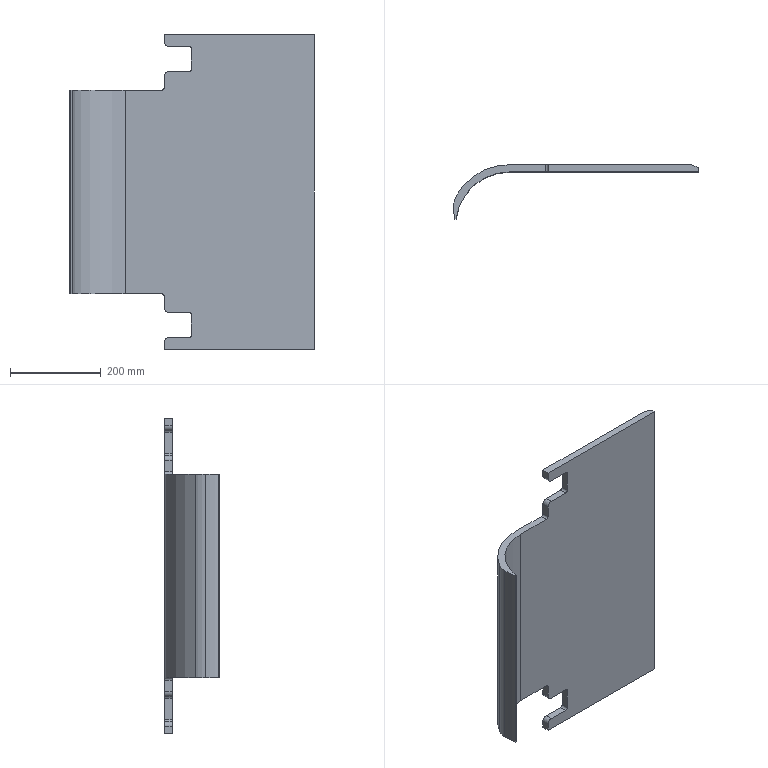Part | SolidWorks | features ICE 2, Extrusion 1 | 1 solid | 33 faces | box 540.8 x 120 x 696 mm | volume 5367152 mm3 | plane 19 | cylinder 14 | commonest cylinder face diameters 10 x6 20 x4 100 x1 236 x1 245.6 x1 268 x1
STEP:
#1=CARTESIAN_POINT('',(418.,9.,-348.));
#2=VERTEX_POINT('',#1);
#3=CARTESIAN_POINT('',(403.,16.,-348.));
#4=VERTEX_POINT('',#3);
#5=CARTESIAN_POINT('',(418.,9.,-348.));
#6=DIRECTION('',(-0.9062,0.4229,0.));
#7=VECTOR('',#6,1000.);
#8=LINE('',#5,#7);
#9=EDGE_CURVE('',#2,#4,#8,.T.);
#10=ORIENTED_EDGE('',*,*,#9,.T.);
#11=CARTESIAN_POINT('',(403.,16.,348.));
#12=VERTEX_POINT('',#11);
#13=CARTESIAN_POINT('',(403.,16.,348.));
#14=DIRECTION('',(0.,0.,-1.));
#15=VECTOR('',#14,1000.);
#16=LINE('',#13,#15);
#17=EDGE_CURVE('',#12,#4,#16,.T.);
#18=ORIENTED_EDGE('',*,*,#17,.F.);
#19=CARTESIAN_POINT('',(418.,9.,348.));
#20=VERTEX_POINT('',#19);
#21=CARTESIAN_POINT('',(418.,9.,348.));
#22=DIRECTION('',(-0.9062,0.4229,0.));
#23=VECTOR('',#22,1000.);
#24=LINE('',#21,#23);
#25=EDGE_CURVE('',#20,#12,#24,.T.);
#26=ORIENTED_EDGE('',*,*,#25,.F.);
#27=CARTESIAN_POINT('',(418.,9.,348.));
#28=DIRECTION('',(0.,0.,-1.));
#29=VECTOR('',#28,1000.);
#30=LINE('',#27,#29);
#31=EDGE_CURVE('',#20,#2,#30,.T.);
#32=ORIENTED_EDGE('',*,*,#31,.T.);
#33=EDGE_LOOP('',(#10,#18,#26,#32));
#34=FACE_OUTER_BOUND('',#33,.T.);
#35=CARTESIAN_POINT('',(418.,9.,348.));
#36=DIRECTION('',(-0.4229,-0.9062,0.));
#37=DIRECTION('',(0.9062,-0.4229,0.));
#38=AXIS2_PLACEMENT_3D('',#35,#36,#37);
#39=PLANE('',#38);
#40=ADVANCED_FACE('',(#34),#39,.F.);
#41=CARTESIAN_POINT('',(0.,16.,225.));
#42=VERTEX_POINT('',#41);
#43=CARTESIAN_POINT('',(0.,16.,-225.));
#44=VERTEX_POINT('',#43);
#45=CARTESIAN_POINT('',(0.,16.,348.));
#46=DIRECTION('',(0.,0.,-1.));
#47=VECTOR('',#46,1000.);
#48=LINE('',#45,#47);
#49=EDGE_CURVE('',#42,#44,#48,.T.);
#50=ORIENTED_EDGE('',*,*,#49,.F.);
#51=CARTESIAN_POINT('',(81.,16.,225.));
#52=VERTEX_POINT('',#51);
#53=CARTESIAN_POINT('',(81.,16.,225.));
#54=DIRECTION('',(-1.,0.,0.));
#55=VECTOR('',#54,1000.);
#56=LINE('',#53,#55);
#57=EDGE_CURVE('',#52,#42,#56,.T.);
#58=ORIENTED_EDGE('',*,*,#57,.F.);
#59=CARTESIAN_POINT('',(86.,16.,230.));
#60=VERTEX_POINT('',#59);
#61=CARTESIAN_POINT('',(81.,16.,230.));
#62=DIRECTION('',(0.,1.,0.));
#63=DIRECTION('',(0.,0.,1.));
#64=AXIS2_PLACEMENT_3D('',#61,#62,#63);
#65=CIRCLE('',#64,5.);
#66=EDGE_CURVE('',#60,#52,#65,.T.);
#67=ORIENTED_EDGE('',*,*,#66,.F.);
#68=CARTESIAN_POINT('',(86.,16.,256.));
#69=VERTEX_POINT('',#68);
#70=CARTESIAN_POINT('',(86.,16.,256.));
#71=DIRECTION('',(0.,0.,-1.));
#72=VECTOR('',#71,1000.);
#73=LINE('',#70,#72);
#74=EDGE_CURVE('',#69,#60,#73,.T.);
#75=ORIENTED_EDGE('',*,*,#74,.F.);
#76=CARTESIAN_POINT('',(96.,16.,266.));
#77=VERTEX_POINT('',#76);
#78=CARTESIAN_POINT('',(96.,16.,256.));
#79=DIRECTION('',(0.,-1.,0.));
#80=DIRECTION('',(0.,0.,-1.));
#81=AXIS2_PLACEMENT_3D('',#78,#79,#80);
#82=CIRCLE('',#81,10.);
#83=EDGE_CURVE('',#77,#69,#82,.T.);
#84=ORIENTED_EDGE('',*,*,#83,.F.);
#85=CARTESIAN_POINT('',(141.,16.,266.));
#86=VERTEX_POINT('',#85);
#87=CARTESIAN_POINT('',(141.,16.,266.));
#88=DIRECTION('',(-1.,0.,0.));
#89=VECTOR('',#88,1000.);
#90=LINE('',#87,#89);
#91=EDGE_CURVE('',#86,#77,#90,.T.);
#92=ORIENTED_EDGE('',*,*,#91,.F.);
#93=CARTESIAN_POINT('',(146.,16.,271.));
#94=VERTEX_POINT('',#93);
#95=CARTESIAN_POINT('',(141.,16.,271.));
#96=DIRECTION('',(0.,1.,0.));
#97=DIRECTION('',(0.,0.,-1.));
#98=AXIS2_PLACEMENT_3D('',#95,#96,#97);
#99=CIRCLE('',#98,5.);
#100=EDGE_CURVE('',#94,#86,#99,.T.);
#101=ORIENTED_EDGE('',*,*,#100,.F.);
#102=CARTESIAN_POINT('',(146.,16.,317.));
#103=VERTEX_POINT('',#102);
#104=CARTESIAN_POINT('',(146.,16.,317.));
#105=DIRECTION('',(0.,0.,-1.));
#106=VECTOR('',#105,1000.);
#107=LINE('',#104,#106);
#108=EDGE_CURVE('',#103,#94,#107,.T.);
#109=ORIENTED_EDGE('',*,*,#108,.F.);
#110=CARTESIAN_POINT('',(141.,16.,322.));
#111=VERTEX_POINT('',#110);
#112=CARTESIAN_POINT('',(141.,16.,317.));
#113=DIRECTION('',(0.,1.,0.));
#114=DIRECTION('',(0.,0.,-1.));
#115=AXIS2_PLACEMENT_3D('',#112,#113,#114);
#116=CIRCLE('',#115,5.);
#117=EDGE_CURVE('',#111,#103,#116,.T.);
#118=ORIENTED_EDGE('',*,*,#117,.F.);
#119=CARTESIAN_POINT('',(96.,16.,322.));
#120=VERTEX_POINT('',#119);
#121=CARTESIAN_POINT('',(96.,16.,322.));
#122=DIRECTION('',(1.,0.,0.));
#123=VECTOR('',#122,1000.);
#124=LINE('',#121,#123);
#125=EDGE_CURVE('',#120,#111,#124,.T.);
#126=ORIENTED_EDGE('',*,*,#125,.F.);
#127=CARTESIAN_POINT('',(86.,16.,332.));
#128=VERTEX_POINT('',#127);
#129=CARTESIAN_POINT('',(96.,16.,332.));
#130=DIRECTION('',(0.,-1.,0.));
#131=DIRECTION('',(0.,0.,1.));
#132=AXIS2_PLACEMENT_3D('',#129,#130,#131);
#133=CIRCLE('',#132,10.);
#134=EDGE_CURVE('',#128,#120,#133,.T.);
#135=ORIENTED_EDGE('',*,*,#134,.F.);
#136=CARTESIAN_POINT('',(86.,16.,348.));
#137=VERTEX_POINT('',#136);
#138=CARTESIAN_POINT('',(86.,16.,332.));
#139=DIRECTION('',(0.,0.,-1.));
#140=VECTOR('',#139,1000.);
#141=LINE('',#138,#140);
#142=EDGE_CURVE('',#137,#128,#141,.T.);
#143=ORIENTED_EDGE('',*,*,#142,.F.);
#144=CARTESIAN_POINT('',(0.,16.,348.));
#145=DIRECTION('',(-1.,0.,0.));
#146=VECTOR('',#145,1000.);
#147=LINE('',#144,#146);
#148=EDGE_CURVE('',#12,#137,#147,.T.);
#149=ORIENTED_EDGE('',*,*,#148,.F.);
#150=ORIENTED_EDGE('',*,*,#17,.T.);
#151=CARTESIAN_POINT('',(86.,16.,-348.));
#152=VERTEX_POINT('',#151);
#153=CARTESIAN_POINT('',(0.,16.,-348.));
#154=DIRECTION('',(-1.,0.,0.));
#155=VECTOR('',#154,1000.);
#156=LINE('',#153,#155);
#157=EDGE_CURVE('',#4,#152,#156,.T.);
#158=ORIENTED_EDGE('',*,*,#157,.T.);
#159=CARTESIAN_POINT('',(86.,16.,-332.));
#160=VERTEX_POINT('',#159);
#161=CARTESIAN_POINT('',(86.,16.,-332.));
#162=DIRECTION('',(0.,0.,-1.));
#163=VECTOR('',#162,1000.);
#164=LINE('',#161,#163);
#165=EDGE_CURVE('',#160,#152,#164,.T.);
#166=ORIENTED_EDGE('',*,*,#165,.F.);
#167=CARTESIAN_POINT('',(96.,16.,-322.));
#168=VERTEX_POINT('',#167);
#169=CARTESIAN_POINT('',(96.,16.,-332.));
#170=DIRECTION('',(0.,-1.,0.));
#171=DIRECTION('',(0.,0.,-1.));
#172=AXIS2_PLACEMENT_3D('',#169,#170,#171);
#173=CIRCLE('',#172,10.);
#174=EDGE_CURVE('',#168,#160,#173,.T.);
#175=ORIENTED_EDGE('',*,*,#174,.F.);
#176=CARTESIAN_POINT('',(141.,16.,-322.));
#177=VERTEX_POINT('',#176);
#178=CARTESIAN_POINT('',(96.,16.,-322.));
#179=DIRECTION('',(-1.,0.,0.));
#180=VECTOR('',#179,1000.);
#181=LINE('',#178,#180);
#182=EDGE_CURVE('',#177,#168,#181,.T.);
#183=ORIENTED_EDGE('',*,*,#182,.F.);
#184=CARTESIAN_POINT('',(146.,16.,-317.));
#185=VERTEX_POINT('',#184);
#186=CARTESIAN_POINT('',(141.,16.,-317.));
#187=DIRECTION('',(0.,1.,0.));
#188=DIRECTION('',(0.,0.,1.));
#189=AXIS2_PLACEMENT_3D('',#186,#187,#188);
#190=CIRCLE('',#189,5.);
#191=EDGE_CURVE('',#185,#177,#190,.T.);
#192=ORIENTED_EDGE('',*,*,#191,.F.);
#193=CARTESIAN_POINT('',(146.,16.,-271.));
#194=VERTEX_POINT('',#193);
#195=CARTESIAN_POINT('',(146.,16.,-317.));
#196=DIRECTION('',(0.,0.,-1.));
#197=VECTOR('',#196,1000.);
#198=LINE('',#195,#197);
#199=EDGE_CURVE('',#194,#185,#198,.T.);
#200=ORIENTED_EDGE('',*,*,#199,.F.);
#201=CARTESIAN_POINT('',(141.,16.,-266.));
#202=VERTEX_POINT('',#201);
#203=CARTESIAN_POINT('',(141.,16.,-271.));
#204=DIRECTION('',(0.,1.,0.));
#205=DIRECTION('',(0.,0.,1.));
#206=AXIS2_PLACEMENT_3D('',#203,#204,#205);
#207=CIRCLE('',#206,5.);
#208=EDGE_CURVE('',#202,#194,#207,.T.);
#209=ORIENTED_EDGE('',*,*,#208,.F.);
#210=CARTESIAN_POINT('',(96.,16.,-266.));
#211=VERTEX_POINT('',#210);
#212=CARTESIAN_POINT('',(141.,16.,-266.));
#213=DIRECTION('',(1.,0.,0.));
#214=VECTOR('',#213,1000.);
#215=LINE('',#212,#214);
#216=EDGE_CURVE('',#211,#202,#215,.T.);
#217=ORIENTED_EDGE('',*,*,#216,.F.);
#218=CARTESIAN_POINT('',(86.,16.,-256.));
#219=VERTEX_POINT('',#218);
#220=CARTESIAN_POINT('',(96.,16.,-256.));
#221=DIRECTION('',(0.,-1.,0.));
#222=DIRECTION('',(0.,0.,1.));
#223=AXIS2_PLACEMENT_3D('',#220,#221,#222);
#224=CIRCLE('',#223,10.);
#225=EDGE_CURVE('',#219,#211,#224,.T.);
#226=ORIENTED_EDGE('',*,*,#225,.F.);
#227=CARTESIAN_POINT('',(86.,16.,-230.));
#228=VERTEX_POINT('',#227);
#229=CARTESIAN_POINT('',(86.,16.,-256.));
#230=DIRECTION('',(0.,0.,-1.));
#231=VECTOR('',#230,1000.);
#232=LINE('',#229,#231);
#233=EDGE_CURVE('',#228,#219,#232,.T.);
#234=ORIENTED_EDGE('',*,*,#233,.F.);
#235=CARTESIAN_POINT('',(81.,16.,-225.));
#236=VERTEX_POINT('',#235);
#237=CARTESIAN_POINT('',(81.,16.,-230.));
#238=DIRECTION('',(0.,1.,0.));
#239=DIRECTION('',(0.,0.,-1.));
#240=AXIS2_PLACEMENT_3D('',#237,#238,#239);
#241=CIRCLE('',#240,5.);
#242=EDGE_CURVE('',#236,#228,#241,.T.);
#243=ORIENTED_EDGE('',*,*,#242,.F.);
#244=CARTESIAN_POINT('',(81.,16.,-225.));
#245=DIRECTION('',(1.,0.,0.));
#246=VECTOR('',#245,1000.);
#247=LINE('',#244,#246);
#248=EDGE_CURVE('',#44,#236,#247,.T.);
#249=ORIENTED_EDGE('',*,*,#248,.F.);
#250=EDGE_LOOP('',(#50,#58,#67,#75,#84,#92,#101,#109,#118,#126,#135,#143,#149,#150,#158,#166,#175,#183,#192,#200,#209,#217,#226,#234,#243,#249));
#251=FACE_OUTER_BOUND('',#250,.T.);
#252=CARTESIAN_POINT('',(0.,16.,348.));
#253=DIRECTION('',(0.,-1.,0.));
#254=DIRECTION('',(1.,0.,0.));
#255=AXIS2_PLACEMENT_3D('',#252,#253,#254);
#256=PLANE('',#255);
#257=ADVANCED_FACE('',(#251),#256,.F.);
#258=CARTESIAN_POINT('',(-116.034,-50.976,-225.));
#259=VERTEX_POINT('',#258);
#260=CARTESIAN_POINT('',(0.,-118.,-225.));
#261=DIRECTION('',(0.,0.,1.));
#262=DIRECTION('',(1.,0.,0.));
#263=AXIS2_PLACEMENT_3D('',#260,#261,#262);
#264=CIRCLE('',#263,134.);
#265=EDGE_CURVE('',#44,#259,#264,.T.);
#266=ORIENTED_EDGE('',*,*,#265,.T.);
#267=CARTESIAN_POINT('',(-116.034,-50.976,225.));
#268=VERTEX_POINT('',#267);
#269=CARTESIAN_POINT('',(-116.034,-50.976,-348.));
#270=DIRECTION('',(0.,0.,1.));
#271=VECTOR('',#270,1000.);
#272=LINE('',#269,#271);
#273=EDGE_CURVE('',#259,#268,#272,.T.);
#274=ORIENTED_EDGE('',*,*,#273,.T.);
#275=CARTESIAN_POINT('',(0.,-118.,225.));
#276=DIRECTION('',(0.,0.,-1.));
#277=DIRECTION('',(-1.,0.,0.));
#278=AXIS2_PLACEMENT_3D('',#275,#276,#277);
#279=CIRCLE('',#278,134.);
#280=EDGE_CURVE('',#268,#42,#279,.T.);
#281=ORIENTED_EDGE('',*,*,#280,.T.);
#282=ORIENTED_EDGE('',*,*,#49,.T.);
#283=EDGE_LOOP('',(#266,#274,#281,#282));
#284=FACE_OUTER_BOUND('',#283,.T.);
#285=CARTESIAN_POINT('',(0.,-118.,348.));
#286=DIRECTION('',(0.,0.,-1.));
#287=DIRECTION('',(-1.,0.,0.));
#288=AXIS2_PLACEMENT_3D('',#285,#286,#287);
#289=CYLINDRICAL_SURFACE('',#288,134.);
#290=ADVANCED_FACE('',(#284),#289,.T.);
#291=CARTESIAN_POINT('',(-117.167,-104.,225.));
#292=VERTEX_POINT('',#291);
#293=CARTESIAN_POINT('',(-120.306,-103.625,225.));
#294=VERTEX_POINT('',#293);
#295=CARTESIAN_POINT('',(-117.167,-104.,225.));
#296=DIRECTION('',(-0.9929,0.1186,0.));
#297=VECTOR('',#296,1000.);
#298=LINE('',#295,#297);
#299=EDGE_CURVE('',#292,#294,#298,.T.);
#300=ORIENTED_EDGE('',*,*,#299,.T.);
#301=CARTESIAN_POINT('',(-120.306,-103.625,-225.));
#302=VERTEX_POINT('',#301);
#303=CARTESIAN_POINT('',(-120.306,-103.625,-348.));
#304=DIRECTION('',(0.,0.,1.));
#305=VECTOR('',#304,1000.);
#306=LINE('',#303,#305);
#307=EDGE_CURVE('',#302,#294,#306,.T.);
#308=ORIENTED_EDGE('',*,*,#307,.F.);
#309=CARTESIAN_POINT('',(-117.167,-104.,-225.));
#310=VERTEX_POINT('',#309);
#311=CARTESIAN_POINT('',(-117.167,-104.,-225.));
#312=DIRECTION('',(0.9929,-0.1186,0.));
#313=VECTOR('',#312,1000.);
#314=LINE('',#311,#313);
#315=EDGE_CURVE('',#302,#310,#314,.T.);
#316=ORIENTED_EDGE('',*,*,#315,.T.);
#317=CARTESIAN_POINT('',(-117.167,-104.,348.));
#318=DIRECTION('',(0.,0.,-1.));
#319=VECTOR('',#318,1000.);
#320=LINE('',#317,#319);
#321=EDGE_CURVE('',#292,#310,#320,.T.);
#322=ORIENTED_EDGE('',*,*,#321,.F.);
#323=EDGE_LOOP('',(#300,#308,#316,#322));
#324=FACE_OUTER_BOUND('',#323,.T.);
#325=CARTESIAN_POINT('',(-117.167,-104.,348.));
#326=DIRECTION('',(0.1186,0.9929,0.));
#327=DIRECTION('',(-0.9929,0.1186,0.));
#328=AXIS2_PLACEMENT_3D('',#325,#326,#327);
#329=PLANE('',#328);
#330=ADVANCED_FACE('',(#324),#329,.F.);
#331=CARTESIAN_POINT('',(0.,0.,225.));
#332=VERTEX_POINT('',#331);
#333=CARTESIAN_POINT('',(0.,0.,-225.));
#334=VERTEX_POINT('',#333);
#335=CARTESIAN_POINT('',(0.,0.,348.));
#336=DIRECTION('',(0.,0.,-1.));
#337=VECTOR('',#336,1000.);
#338=LINE('',#335,#337);
#339=EDGE_CURVE('',#332,#334,#338,.T.);
#340=ORIENTED_EDGE('',*,*,#339,.F.);
#341=CARTESIAN_POINT('',(0.,-118.,225.));
#342=DIRECTION('',(0.,0.,1.));
#343=DIRECTION('',(-1.,0.,0.));
#344=AXIS2_PLACEMENT_3D('',#341,#342,#343);
#345=CIRCLE('',#344,118.);
#346=EDGE_CURVE('',#332,#292,#345,.T.);
#347=ORIENTED_EDGE('',*,*,#346,.T.);
#348=ORIENTED_EDGE('',*,*,#321,.T.);
#349=CARTESIAN_POINT('',(0.,-118.,-225.));
#350=DIRECTION('',(0.,0.,-1.));
#351=DIRECTION('',(1.,0.,0.));
#352=AXIS2_PLACEMENT_3D('',#349,#350,#351);
#353=CIRCLE('',#352,118.);
#354=EDGE_CURVE('',#310,#334,#353,.T.);
#355=ORIENTED_EDGE('',*,*,#354,.T.);
#356=EDGE_LOOP('',(#340,#347,#348,#355));
#357=FACE_OUTER_BOUND('',#356,.T.);
#358=CARTESIAN_POINT('',(0.,-118.,348.));
#359=DIRECTION('',(0.,0.,-1.));
#360=DIRECTION('',(-1.,0.,0.));
#361=AXIS2_PLACEMENT_3D('',#358,#359,#360);
#362=CYLINDRICAL_SURFACE('',#361,118.);
#363=ADVANCED_FACE('',(#357),#362,.F.);
#364=CARTESIAN_POINT('',(86.,0.,230.));
#365=VERTEX_POINT('',#364);
#366=CARTESIAN_POINT('',(81.,0.,225.));
#367=VERTEX_POINT('',#366);
#368=CARTESIAN_POINT('',(81.,0.,230.));
#369=DIRECTION('',(0.,1.,0.));
#370=DIRECTION('',(0.,0.,1.));
#371=AXIS2_PLACEMENT_3D('',#368,#369,#370);
#372=CIRCLE('',#371,5.);
#373=EDGE_CURVE('',#365,#367,#372,.T.);
#374=ORIENTED_EDGE('',*,*,#373,.T.);
#375=CARTESIAN_POINT('',(0.,0.,225.));
#376=DIRECTION('',(-1.,0.,0.));
#377=VECTOR('',#376,1000.);
#378=LINE('',#375,#377);
#379=EDGE_CURVE('',#367,#332,#378,.T.);
#380=ORIENTED_EDGE('',*,*,#379,.T.);
#381=ORIENTED_EDGE('',*,*,#339,.T.);
#382=CARTESIAN_POINT('',(81.,0.,-225.));
#383=VERTEX_POINT('',#382);
#384=CARTESIAN_POINT('',(0.,0.,-225.));
#385=DIRECTION('',(1.,0.,0.));
#386=VECTOR('',#385,1000.);
#387=LINE('',#384,#386);
#388=EDGE_CURVE('',#334,#383,#387,.T.);
#389=ORIENTED_EDGE('',*,*,#388,.T.);
#390=CARTESIAN_POINT('',(86.,0.,-230.));
#391=VERTEX_POINT('',#390);
#392=CARTESIAN_POINT('',(81.,0.,-230.));
#393=DIRECTION('',(0.,1.,0.));
#394=DIRECTION('',(0.,0.,1.));
#395=AXIS2_PLACEMENT_3D('',#392,#393,#394);
#396=CIRCLE('',#395,5.);
#397=EDGE_CURVE('',#383,#391,#396,.T.);
#398=ORIENTED_EDGE('',*,*,#397,.T.);
#399=CARTESIAN_POINT('',(86.,0.,-256.));
#400=VERTEX_POINT('',#399);
#401=CARTESIAN_POINT('',(86.,0.,348.));
#402=DIRECTION('',(0.,0.,-1.));
#403=VECTOR('',#402,1000.);
#404=LINE('',#401,#403);
#405=EDGE_CURVE('',#391,#400,#404,.T.);
#406=ORIENTED_EDGE('',*,*,#405,.T.);
#407=CARTESIAN_POINT('',(96.,0.,-266.));
#408=VERTEX_POINT('',#407);
#409=CARTESIAN_POINT('',(96.,0.,-256.));
#410=DIRECTION('',(0.,-1.,0.));
#411=DIRECTION('',(0.,0.,1.));
#412=AXIS2_PLACEMENT_3D('',#409,#410,#411);
#413=CIRCLE('',#412,10.);
#414=EDGE_CURVE('',#400,#408,#413,.T.);
#415=ORIENTED_EDGE('',*,*,#414,.T.);
#416=CARTESIAN_POINT('',(141.,0.,-266.));
#417=VERTEX_POINT('',#416);
#418=CARTESIAN_POINT('',(0.,0.,-266.));
#419=DIRECTION('',(1.,0.,0.));
#420=VECTOR('',#419,1000.);
#421=LINE('',#418,#420);
#422=EDGE_CURVE('',#408,#417,#421,.T.);
#423=ORIENTED_EDGE('',*,*,#422,.T.);
#424=CARTESIAN_POINT('',(146.,0.,-271.));
#425=VERTEX_POINT('',#424);
#426=CARTESIAN_POINT('',(141.,0.,-271.));
#427=DIRECTION('',(0.,1.,0.));
#428=DIRECTION('',(0.,0.,1.));
#429=AXIS2_PLACEMENT_3D('',#426,#427,#428);
#430=CIRCLE('',#429,5.);
#431=EDGE_CURVE('',#417,#425,#430,.T.);
#432=ORIENTED_EDGE('',*,*,#431,.T.);
#433=CARTESIAN_POINT('',(146.,0.,-317.));
#434=VERTEX_POINT('',#433);
#435=CARTESIAN_POINT('',(146.,0.,348.));
#436=DIRECTION('',(0.,0.,-1.));
#437=VECTOR('',#436,1000.);
#438=LINE('',#435,#437);
#439=EDGE_CURVE('',#425,#434,#438,.T.);
#440=ORIENTED_EDGE('',*,*,#439,.T.);
#441=CARTESIAN_POINT('',(141.,0.,-322.));
#442=VERTEX_POINT('',#441);
#443=CARTESIAN_POINT('',(141.,0.,-317.));
#444=DIRECTION('',(0.,1.,0.));
#445=DIRECTION('',(0.,0.,1.));
#446=AXIS2_PLACEMENT_3D('',#443,#444,#445);
#447=CIRCLE('',#446,5.);
#448=EDGE_CURVE('',#434,#442,#447,.T.);
#449=ORIENTED_EDGE('',*,*,#448,.T.);
#450=CARTESIAN_POINT('',(96.,0.,-322.));
#451=VERTEX_POINT('',#450);
#452=CARTESIAN_POINT('',(0.,0.,-322.));
#453=DIRECTION('',(-1.,0.,0.));
#454=VECTOR('',#453,1000.);
#455=LINE('',#452,#454);
#456=EDGE_CURVE('',#442,#451,#455,.T.);
#457=ORIENTED_EDGE('',*,*,#456,.T.);
#458=CARTESIAN_POINT('',(86.,0.,-332.));
#459=VERTEX_POINT('',#458);
#460=CARTESIAN_POINT('',(96.,0.,-332.));
#461=DIRECTION('',(0.,-1.,0.));
#462=DIRECTION('',(0.,0.,1.));
#463=AXIS2_PLACEMENT_3D('',#460,#461,#462);
#464=CIRCLE('',#463,10.);
#465=EDGE_CURVE('',#451,#459,#464,.T.);
#466=ORIENTED_EDGE('',*,*,#465,.T.);
#467=CARTESIAN_POINT('',(86.,0.,-348.));
#468=VERTEX_POINT('',#467);
#469=CARTESIAN_POINT('',(86.,0.,348.));
#470=DIRECTION('',(0.,0.,-1.));
#471=VECTOR('',#470,1000.);
#472=LINE('',#469,#471);
#473=EDGE_CURVE('',#459,#468,#472,.T.);
#474=ORIENTED_EDGE('',*,*,#473,.T.);
#475=CARTESIAN_POINT('',(418.,0.,-348.));
#476=VERTEX_POINT('',#475);
#477=CARTESIAN_POINT('',(0.,0.,-348.));
#478=DIRECTION('',(1.,0.,0.));
#479=VECTOR('',#478,1000.);
#480=LINE('',#477,#479);
#481=EDGE_CURVE('',#468,#476,#480,.T.);
#482=ORIENTED_EDGE('',*,*,#481,.T.);
#483=CARTESIAN_POINT('',(418.,0.,348.));
#484=VERTEX_POINT('',#483);
#485=CARTESIAN_POINT('',(418.,0.,348.));
#486=DIRECTION('',(0.,0.,-1.));
#487=VECTOR('',#486,1000.);
#488=LINE('',#485,#487);
#489=EDGE_CURVE('',#484,#476,#488,.T.);
#490=ORIENTED_EDGE('',*,*,#489,.F.);
#491=CARTESIAN_POINT('',(86.,0.,348.));
#492=VERTEX_POINT('',#491);
#493=CARTESIAN_POINT('',(0.,0.,348.));
#494=DIRECTION('',(1.,0.,0.));
#495=VECTOR('',#494,1000.);
#496=LINE('',#493,#495);
#497=EDGE_CURVE('',#492,#484,#496,.T.);
#498=ORIENTED_EDGE('',*,*,#497,.F.);
#499=CARTESIAN_POINT('',(86.,0.,332.));
#500=VERTEX_POINT('',#499);
#501=CARTESIAN_POINT('',(86.,0.,348.));
#502=DIRECTION('',(0.,0.,-1.));
#503=VECTOR('',#502,1000.);
#504=LINE('',#501,#503);
#505=EDGE_CURVE('',#492,#500,#504,.T.);
#506=ORIENTED_EDGE('',*,*,#505,.T.);
#507=CARTESIAN_POINT('',(96.,0.,322.));
#508=VERTEX_POINT('',#507);
#509=CARTESIAN_POINT('',(96.,0.,332.));
#510=DIRECTION('',(0.,-1.,0.));
#511=DIRECTION('',(0.,0.,1.));
#512=AXIS2_PLACEMENT_3D('',#509,#510,#511);
#513=CIRCLE('',#512,10.);
#514=EDGE_CURVE('',#500,#508,#513,.T.);
#515=ORIENTED_EDGE('',*,*,#514,.T.);
#516=CARTESIAN_POINT('',(141.,0.,322.));
#517=VERTEX_POINT('',#516);
#518=CARTESIAN_POINT('',(0.,0.,322.));
#519=DIRECTION('',(1.,0.,0.));
#520=VECTOR('',#519,1000.);
#521=LINE('',#518,#520);
#522=EDGE_CURVE('',#508,#517,#521,.T.);
#523=ORIENTED_EDGE('',*,*,#522,.T.);
#524=CARTESIAN_POINT('',(146.,0.,317.));
#525=VERTEX_POINT('',#524);
#526=CARTESIAN_POINT('',(141.,0.,317.));
#527=DIRECTION('',(0.,1.,0.));
#528=DIRECTION('',(0.,0.,1.));
#529=AXIS2_PLACEMENT_3D('',#526,#527,#528);
#530=CIRCLE('',#529,5.);
#531=EDGE_CURVE('',#517,#525,#530,.T.);
#532=ORIENTED_EDGE('',*,*,#531,.T.);
#533=CARTESIAN_POINT('',(146.,0.,271.));
#534=VERTEX_POINT('',#533);
#535=CARTESIAN_POINT('',(146.,0.,348.));
#536=DIRECTION('',(0.,0.,-1.));
#537=VECTOR('',#536,1000.);
#538=LINE('',#535,#537);
#539=EDGE_CURVE('',#525,#534,#538,.T.);
#540=ORIENTED_EDGE('',*,*,#539,.T.);
#541=CARTESIAN_POINT('',(141.,0.,266.));
#542=VERTEX_POINT('',#541);
#543=CARTESIAN_POINT('',(141.,0.,271.));
#544=DIRECTION('',(0.,1.,0.));
#545=DIRECTION('',(0.,0.,1.));
#546=AXIS2_PLACEMENT_3D('',#543,#544,#545);
#547=CIRCLE('',#546,5.);
#548=EDGE_CURVE('',#534,#542,#547,.T.);
#549=ORIENTED_EDGE('',*,*,#548,.T.);
#550=CARTESIAN_POINT('',(96.,0.,266.));
#551=VERTEX_POINT('',#550);
#552=CARTESIAN_POINT('',(0.,0.,266.));
#553=DIRECTION('',(-1.,0.,0.));
#554=VECTOR('',#553,1000.);
#555=LINE('',#552,#554);
#556=EDGE_CURVE('',#542,#551,#555,.T.);
#557=ORIENTED_EDGE('',*,*,#556,.T.);
#558=CARTESIAN_POINT('',(86.,0.,256.));
#559=VERTEX_POINT('',#558);
#560=CARTESIAN_POINT('',(96.,0.,256.));
#561=DIRECTION('',(0.,-1.,0.));
#562=DIRECTION('',(0.,0.,1.));
#563=AXIS2_PLACEMENT_3D('',#560,#561,#562);
#564=CIRCLE('',#563,10.);
#565=EDGE_CURVE('',#551,#559,#564,.T.);
#566=ORIENTED_EDGE('',*,*,#565,.T.);
#567=CARTESIAN_POINT('',(86.,0.,348.));
#568=DIRECTION('',(0.,0.,-1.));
#569=VECTOR('',#568,1000.);
#570=LINE('',#567,#569);
#571=EDGE_CURVE('',#559,#365,#570,.T.);
#572=ORIENTED_EDGE('',*,*,#571,.T.);
#573=EDGE_LOOP('',(#374,#380,#381,#389,#398,#406,#415,#423,#432,#440,#449,#457,#466,#474,#482,#490,#498,#506,#515,#523,#532,#540,#549,#557,#566,#572));
#574=FACE_OUTER_BOUND('',#573,.T.);
#575=CARTESIAN_POINT('',(0.,0.,348.));
#576=DIRECTION('',(0.,1.,0.));
#577=DIRECTION('',(0.,0.,1.));
#578=AXIS2_PLACEMENT_3D('',#575,#576,#577);
#579=PLANE('',#578);
#580=ADVANCED_FACE('',(#574),#579,.F.);
#581=CARTESIAN_POINT('',(418.,0.,-348.));
#582=DIRECTION('',(0.,1.,0.));
#583=VECTOR('',#582,1000.);
#584=LINE('',#581,#583);
#585=EDGE_CURVE('',#476,#2,#584,.T.);
#586=ORIENTED_EDGE('',*,*,#585,.T.);
#587=ORIENTED_EDGE('',*,*,#31,.F.);
#588=CARTESIAN_POINT('',(418.,0.,348.));
#589=DIRECTION('',(0.,1.,0.));
#590=VECTOR('',#589,1000.);
#591=LINE('',#588,#590);
#592=EDGE_CURVE('',#484,#20,#591,.T.);
#593=ORIENTED_EDGE('',*,*,#592,.F.);
#594=ORIENTED_EDGE('',*,*,#489,.T.);
#595=EDGE_LOOP('',(#586,#587,#593,#594));
#596=FACE_OUTER_BOUND('',#595,.T.);
#597=CARTESIAN_POINT('',(418.,0.,348.));
#598=DIRECTION('',(-1.,0.,0.));
#599=DIRECTION('',(0.,0.,1.));
#600=AXIS2_PLACEMENT_3D('',#597,#598,#599);
#601=PLANE('',#600);
#602=ADVANCED_FACE('',(#596),#601,.F.);
#603=CARTESIAN_POINT('',(86.,-118.,348.));
#604=DIRECTION('',(0.,1.,0.));
#605=VECTOR('',#604,1000.);
#606=LINE('',#603,#605);
#607=EDGE_CURVE('',#492,#137,#606,.T.);
#608=ORIENTED_EDGE('',*,*,#607,.F.);
#609=ORIENTED_EDGE('',*,*,#497,.T.);
#610=ORIENTED_EDGE('',*,*,#592,.T.);
#611=ORIENTED_EDGE('',*,*,#25,.T.);
#612=ORIENTED_EDGE('',*,*,#148,.T.);
#613=EDGE_LOOP('',(#608,#609,#610,#611,#612));
#614=FACE_OUTER_BOUND('',#613,.T.);
#615=CARTESIAN_POINT('',(0.,-118.,348.));
#616=DIRECTION('',(0.,0.,1.));
#617=DIRECTION('',(1.,0.,0.));
#618=AXIS2_PLACEMENT_3D('',#615,#616,#617);
#619=PLANE('',#618);
#620=ADVANCED_FACE('',(#614),#619,.T.);
#621=ORIENTED_EDGE('',*,*,#481,.F.);
#622=CARTESIAN_POINT('',(86.,-118.,-348.));
#623=DIRECTION('',(0.,1.,0.));
#624=VECTOR('',#623,1000.);
#625=LINE('',#622,#624);
#626=EDGE_CURVE('',#468,#152,#625,.T.);
#627=ORIENTED_EDGE('',*,*,#626,.T.);
#628=ORIENTED_EDGE('',*,*,#157,.F.);
#629=ORIENTED_EDGE('',*,*,#9,.F.);
#630=ORIENTED_EDGE('',*,*,#585,.F.);
#631=EDGE_LOOP('',(#621,#627,#628,#629,#630));
#632=FACE_OUTER_BOUND('',#631,.T.);
#633=CARTESIAN_POINT('',(0.,-118.,-348.));
#634=DIRECTION('',(0.,0.,1.));
#635=DIRECTION('',(1.,0.,0.));
#636=AXIS2_PLACEMENT_3D('',#633,#634,#635);
#637=PLANE('',#636);
#638=ADVANCED_FACE('',(#632),#637,.F.);
#639=CARTESIAN_POINT('',(96.,-104.,-322.));
#640=DIRECTION('',(0.,1.,0.));
#641=VECTOR('',#640,1000.);
#642=LINE('',#639,#641);
#643=EDGE_CURVE('',#451,#168,#642,.T.);
#644=ORIENTED_EDGE('',*,*,#643,.T.);
#645=ORIENTED_EDGE('',*,*,#174,.T.);
#646=CARTESIAN_POINT('',(86.,-104.,-332.));
#647=DIRECTION('',(0.,1.,0.));
#648=VECTOR('',#647,1000.);
#649=LINE('',#646,#648);
#650=EDGE_CURVE('',#459,#160,#649,.T.);
#651=ORIENTED_EDGE('',*,*,#650,.F.);
#652=ORIENTED_EDGE('',*,*,#465,.F.);
#653=EDGE_LOOP('',(#644,#645,#651,#652));
#654=FACE_OUTER_BOUND('',#653,.T.);
#655=CARTESIAN_POINT('',(96.,-104.,-332.));
#656=DIRECTION('',(0.,1.,0.));
#657=DIRECTION('',(0.,0.,1.));
#658=AXIS2_PLACEMENT_3D('',#655,#656,#657);
#659=CYLINDRICAL_SURFACE('',#658,10.);
#660=ADVANCED_FACE('',(#654),#659,.T.);
#661=CARTESIAN_POINT('',(141.,-104.,-322.));
#662=DIRECTION('',(0.,1.,0.));
#663=VECTOR('',#662,1000.);
#664=LINE('',#661,#663);
#665=EDGE_CURVE('',#442,#177,#664,.T.);
#666=ORIENTED_EDGE('',*,*,#665,.T.);
#667=ORIENTED_EDGE('',*,*,#182,.T.);
#668=ORIENTED_EDGE('',*,*,#643,.F.);
#669=ORIENTED_EDGE('',*,*,#456,.F.);
#670=EDGE_LOOP('',(#666,#667,#668,#669));
#671=FACE_OUTER_BOUND('',#670,.T.);
#672=CARTESIAN_POINT('',(96.,-104.,-322.));
#673=DIRECTION('',(0.,0.,-1.));
#674=DIRECTION('',(-1.,0.,0.));
#675=AXIS2_PLACEMENT_3D('',#672,#673,#674);
#676=PLANE('',#675);
#677=ADVANCED_FACE('',(#671),#676,.F.);
#678=CARTESIAN_POINT('',(146.,-104.,-317.));
#679=DIRECTION('',(0.,1.,0.));
#680=VECTOR('',#679,1000.);
#681=LINE('',#678,#680);
#682=EDGE_CURVE('',#434,#185,#681,.T.);
#683=ORIENTED_EDGE('',*,*,#682,.T.);
#684=ORIENTED_EDGE('',*,*,#191,.T.);
#685=ORIENTED_EDGE('',*,*,#665,.F.);
#686=ORIENTED_EDGE('',*,*,#448,.F.);
#687=EDGE_LOOP('',(#683,#684,#685,#686));
#688=FACE_OUTER_BOUND('',#687,.T.);
#689=CARTESIAN_POINT('',(141.,-104.,-317.));
#690=DIRECTION('',(0.,1.,0.));
#691=DIRECTION('',(0.,0.,1.));
#692=AXIS2_PLACEMENT_3D('',#689,#690,#691);
#693=CYLINDRICAL_SURFACE('',#692,5.);
#694=ADVANCED_FACE('',(#688),#693,.F.);
#695=CARTESIAN_POINT('',(146.,-104.,-271.));
#696=DIRECTION('',(0.,1.,0.));
#697=VECTOR('',#696,1000.);
#698=LINE('',#695,#697);
#699=EDGE_CURVE('',#425,#194,#698,.T.);
#700=ORIENTED_EDGE('',*,*,#699,.T.);
#701=ORIENTED_EDGE('',*,*,#199,.T.);
#702=ORIENTED_EDGE('',*,*,#682,.F.);
#703=ORIENTED_EDGE('',*,*,#439,.F.);
#704=EDGE_LOOP('',(#700,#701,#702,#703));
#705=FACE_OUTER_BOUND('',#704,.T.);
#706=CARTESIAN_POINT('',(146.,-104.,-317.));
#707=DIRECTION('',(1.,0.,0.));
#708=DIRECTION('',(0.,0.,-1.));
#709=AXIS2_PLACEMENT_3D('',#706,#707,#708);
#710=PLANE('',#709);
#711=ADVANCED_FACE('',(#705),#710,.F.);
#712=CARTESIAN_POINT('',(141.,-104.,-266.));
#713=DIRECTION('',(0.,1.,0.));
#714=VECTOR('',#713,1000.);
#715=LINE('',#712,#714);
#716=EDGE_CURVE('',#417,#202,#715,.T.);
#717=ORIENTED_EDGE('',*,*,#716,.T.);
#718=ORIENTED_EDGE('',*,*,#208,.T.);
#719=ORIENTED_EDGE('',*,*,#699,.F.);
#720=ORIENTED_EDGE('',*,*,#431,.F.);
#721=EDGE_LOOP('',(#717,#718,#719,#720));
#722=FACE_OUTER_BOUND('',#721,.T.);
#723=CARTESIAN_POINT('',(141.,-104.,-271.));
#724=DIRECTION('',(0.,1.,0.));
#725=DIRECTION('',(0.,0.,1.));
#726=AXIS2_PLACEMENT_3D('',#723,#724,#725);
#727=CYLINDRICAL_SURFACE('',#726,5.);
#728=ADVANCED_FACE('',(#722),#727,.F.);
#729=CARTESIAN_POINT('',(96.,-104.,-266.));
#730=DIRECTION('',(0.,1.,0.));
#731=VECTOR('',#730,1000.);
#732=LINE('',#729,#731);
#733=EDGE_CURVE('',#408,#211,#732,.T.);
#734=ORIENTED_EDGE('',*,*,#733,.T.);
#735=ORIENTED_EDGE('',*,*,#216,.T.);
#736=ORIENTED_EDGE('',*,*,#716,.F.);
#737=ORIENTED_EDGE('',*,*,#422,.F.);
#738=EDGE_LOOP('',(#734,#735,#736,#737));
#739=FACE_OUTER_BOUND('',#738,.T.);
#740=CARTESIAN_POINT('',(141.,-104.,-266.));
#741=DIRECTION('',(0.,0.,1.));
#742=DIRECTION('',(1.,0.,0.));
#743=AXIS2_PLACEMENT_3D('',#740,#741,#742);
#744=PLANE('',#743);
#745=ADVANCED_FACE('',(#739),#744,.F.);
#746=CARTESIAN_POINT('',(86.,-104.,-256.));
#747=DIRECTION('',(0.,1.,0.));
#748=VECTOR('',#747,1000.);
#749=LINE('',#746,#748);
#750=EDGE_CURVE('',#400,#219,#749,.T.);
#751=ORIENTED_EDGE('',*,*,#750,.T.);
#752=ORIENTED_EDGE('',*,*,#225,.T.);
#753=ORIENTED_EDGE('',*,*,#733,.F.);
#754=ORIENTED_EDGE('',*,*,#414,.F.);
#755=EDGE_LOOP('',(#751,#752,#753,#754));
#756=FACE_OUTER_BOUND('',#755,.T.);
#757=CARTESIAN_POINT('',(96.,-104.,-256.));
#758=DIRECTION('',(0.,1.,0.));
#759=DIRECTION('',(0.,0.,1.));
#760=AXIS2_PLACEMENT_3D('',#757,#758,#759);
#761=CYLINDRICAL_SURFACE('',#760,10.);
#762=ADVANCED_FACE('',(#756),#761,.T.);
#763=CARTESIAN_POINT('',(86.,-104.,-230.));
#764=DIRECTION('',(0.,1.,0.));
#765=VECTOR('',#764,1000.);
#766=LINE('',#763,#765);
#767=EDGE_CURVE('',#391,#228,#766,.T.);
#768=ORIENTED_EDGE('',*,*,#767,.T.);
#769=ORIENTED_EDGE('',*,*,#233,.T.);
#770=ORIENTED_EDGE('',*,*,#750,.F.);
#771=ORIENTED_EDGE('',*,*,#405,.F.);
#772=EDGE_LOOP('',(#768,#769,#770,#771));
#773=FACE_OUTER_BOUND('',#772,.T.);
#774=CARTESIAN_POINT('',(86.,-104.,-256.));
#775=DIRECTION('',(1.,0.,0.));
#776=DIRECTION('',(0.,0.,-1.));
#777=AXIS2_PLACEMENT_3D('',#774,#775,#776);
#778=PLANE('',#777);
#779=ADVANCED_FACE('',(#773),#778,.F.);
#780=CARTESIAN_POINT('',(81.,-104.,-225.));
#781=DIRECTION('',(0.,1.,0.));
#782=VECTOR('',#781,1000.);
#783=LINE('',#780,#782);
#784=EDGE_CURVE('',#383,#236,#783,.T.);
#785=ORIENTED_EDGE('',*,*,#784,.T.);
#786=ORIENTED_EDGE('',*,*,#242,.T.);
#787=ORIENTED_EDGE('',*,*,#767,.F.);
#788=ORIENTED_EDGE('',*,*,#397,.F.);
#789=EDGE_LOOP('',(#785,#786,#787,#788));
#790=FACE_OUTER_BOUND('',#789,.T.);
#791=CARTESIAN_POINT('',(81.,-104.,-230.));
#792=DIRECTION('',(0.,1.,0.));
#793=DIRECTION('',(0.,0.,1.));
#794=AXIS2_PLACEMENT_3D('',#791,#792,#793);
#795=CYLINDRICAL_SURFACE('',#794,5.);
#796=ADVANCED_FACE('',(#790),#795,.F.);
#797=ORIENTED_EDGE('',*,*,#315,.F.);
#798=CARTESIAN_POINT('',(-122.695,-73.914,-225.));
#799=VERTEX_POINT('',#798);
#800=CARTESIAN_POINT('',(0.,-79.,-225.));
#801=DIRECTION('',(0.,0.,-1.));
#802=DIRECTION('',(1.,0.,0.));
#803=AXIS2_PLACEMENT_3D('',#800,#801,#802);
#804=CIRCLE('',#803,122.8);
#805=EDGE_CURVE('',#302,#799,#804,.T.);
#806=ORIENTED_EDGE('',*,*,#805,.T.);
#807=CARTESIAN_POINT('',(-72.738,-75.985,-225.));
#808=DIRECTION('',(0.,0.,-1.));
#809=DIRECTION('',(1.,0.,0.));
#810=AXIS2_PLACEMENT_3D('',#807,#808,#809);
#811=CIRCLE('',#810,50.);
#812=EDGE_CURVE('',#799,#259,#811,.T.);
#813=ORIENTED_EDGE('',*,*,#812,.T.);
#814=ORIENTED_EDGE('',*,*,#265,.F.);
#815=ORIENTED_EDGE('',*,*,#248,.T.);
#816=ORIENTED_EDGE('',*,*,#784,.F.);
#817=ORIENTED_EDGE('',*,*,#388,.F.);
#818=ORIENTED_EDGE('',*,*,#354,.F.);
#819=EDGE_LOOP('',(#797,#806,#813,#814,#815,#816,#817,#818));
#820=FACE_OUTER_BOUND('',#819,.T.);
#821=CARTESIAN_POINT('',(81.,-104.,-225.));
#822=DIRECTION('',(0.,0.,1.));
#823=DIRECTION('',(1.,0.,0.));
#824=AXIS2_PLACEMENT_3D('',#821,#822,#823);
#825=PLANE('',#824);
#826=ADVANCED_FACE('',(#820),#825,.F.);
#827=ORIENTED_EDGE('',*,*,#650,.T.);
#828=ORIENTED_EDGE('',*,*,#165,.T.);
#829=ORIENTED_EDGE('',*,*,#626,.F.);
#830=ORIENTED_EDGE('',*,*,#473,.F.);
#831=EDGE_LOOP('',(#827,#828,#829,#830));
#832=FACE_OUTER_BOUND('',#831,.T.);
#833=CARTESIAN_POINT('',(86.,-104.,-332.));
#834=DIRECTION('',(1.,0.,0.));
#835=DIRECTION('',(0.,0.,-1.));
#836=AXIS2_PLACEMENT_3D('',#833,#834,#835);
#837=PLANE('',#836);
#838=ADVANCED_FACE('',(#832),#837,.F.);
#839=CARTESIAN_POINT('',(-122.695,-73.914,225.));
#840=VERTEX_POINT('',#839);
#841=CARTESIAN_POINT('',(-72.738,-75.985,225.));
#842=DIRECTION('',(0.,0.,-1.));
#843=DIRECTION('',(1.,0.,0.));
#844=AXIS2_PLACEMENT_3D('',#841,#842,#843);
#845=CIRCLE('',#844,50.);
#846=EDGE_CURVE('',#840,#268,#845,.T.);
#847=ORIENTED_EDGE('',*,*,#846,.F.);
#848=CARTESIAN_POINT('',(0.,-79.,225.));
#849=DIRECTION('',(0.,0.,-1.));
#850=DIRECTION('',(1.,0.,0.));
#851=AXIS2_PLACEMENT_3D('',#848,#849,#850);
#852=CIRCLE('',#851,122.8);
#853=EDGE_CURVE('',#294,#840,#852,.T.);
#854=ORIENTED_EDGE('',*,*,#853,.F.);
#855=ORIENTED_EDGE('',*,*,#299,.F.);
#856=ORIENTED_EDGE('',*,*,#346,.F.);
#857=ORIENTED_EDGE('',*,*,#379,.F.);
#858=CARTESIAN_POINT('',(81.,-104.,225.));
#859=DIRECTION('',(0.,1.,0.));
#860=VECTOR('',#859,1000.);
#861=LINE('',#858,#860);
#862=EDGE_CURVE('',#367,#52,#861,.T.);
#863=ORIENTED_EDGE('',*,*,#862,.T.);
#864=ORIENTED_EDGE('',*,*,#57,.T.);
#865=ORIENTED_EDGE('',*,*,#280,.F.);
#866=EDGE_LOOP('',(#847,#854,#855,#856,#857,#863,#864,#865));
#867=FACE_OUTER_BOUND('',#866,.T.);
#868=CARTESIAN_POINT('',(81.,-104.,225.));
#869=DIRECTION('',(0.,0.,-1.));
#870=DIRECTION('',(-1.,0.,0.));
#871=AXIS2_PLACEMENT_3D('',#868,#869,#870);
#872=PLANE('',#871);
#873=ADVANCED_FACE('',(#867),#872,.F.);
#874=CARTESIAN_POINT('',(86.,-104.,230.));
#875=DIRECTION('',(0.,1.,0.));
#876=VECTOR('',#875,1000.);
#877=LINE('',#874,#876);
#878=EDGE_CURVE('',#365,#60,#877,.T.);
#879=ORIENTED_EDGE('',*,*,#878,.T.);
#880=ORIENTED_EDGE('',*,*,#66,.T.);
#881=ORIENTED_EDGE('',*,*,#862,.F.);
#882=ORIENTED_EDGE('',*,*,#373,.F.);
#883=EDGE_LOOP('',(#879,#880,#881,#882));
#884=FACE_OUTER_BOUND('',#883,.T.);
#885=CARTESIAN_POINT('',(81.,-104.,230.));
#886=DIRECTION('',(0.,1.,0.));
#887=DIRECTION('',(0.,0.,1.));
#888=AXIS2_PLACEMENT_3D('',#885,#886,#887);
#889=CYLINDRICAL_SURFACE('',#888,5.);
#890=ADVANCED_FACE('',(#884),#889,.F.);
#891=CARTESIAN_POINT('',(86.,-104.,256.));
#892=DIRECTION('',(0.,1.,0.));
#893=VECTOR('',#892,1000.);
#894=LINE('',#891,#893);
#895=EDGE_CURVE('',#559,#69,#894,.T.);
#896=ORIENTED_EDGE('',*,*,#895,.T.);
#897=ORIENTED_EDGE('',*,*,#74,.T.);
#898=ORIENTED_EDGE('',*,*,#878,.F.);
#899=ORIENTED_EDGE('',*,*,#571,.F.);
#900=EDGE_LOOP('',(#896,#897,#898,#899));
#901=FACE_OUTER_BOUND('',#900,.T.);
#902=CARTESIAN_POINT('',(86.,-104.,256.));
#903=DIRECTION('',(1.,0.,0.));
#904=DIRECTION('',(0.,0.,-1.));
#905=AXIS2_PLACEMENT_3D('',#902,#903,#904);
#906=PLANE('',#905);
#907=ADVANCED_FACE('',(#901),#906,.F.);
#908=CARTESIAN_POINT('',(96.,-104.,266.));
#909=DIRECTION('',(0.,1.,0.));
#910=VECTOR('',#909,1000.);
#911=LINE('',#908,#910);
#912=EDGE_CURVE('',#551,#77,#911,.T.);
#913=ORIENTED_EDGE('',*,*,#912,.T.);
#914=ORIENTED_EDGE('',*,*,#83,.T.);
#915=ORIENTED_EDGE('',*,*,#895,.F.);
#916=ORIENTED_EDGE('',*,*,#565,.F.);
#917=EDGE_LOOP('',(#913,#914,#915,#916));
#918=FACE_OUTER_BOUND('',#917,.T.);
#919=CARTESIAN_POINT('',(96.,-104.,256.));
#920=DIRECTION('',(0.,1.,0.));
#921=DIRECTION('',(0.,0.,1.));
#922=AXIS2_PLACEMENT_3D('',#919,#920,#921);
#923=CYLINDRICAL_SURFACE('',#922,10.);
#924=ADVANCED_FACE('',(#918),#923,.T.);
#925=CARTESIAN_POINT('',(141.,-104.,266.));
#926=DIRECTION('',(0.,1.,0.));
#927=VECTOR('',#926,1000.);
#928=LINE('',#925,#927);
#929=EDGE_CURVE('',#542,#86,#928,.T.);
#930=ORIENTED_EDGE('',*,*,#929,.T.);
#931=ORIENTED_EDGE('',*,*,#91,.T.);
#932=ORIENTED_EDGE('',*,*,#912,.F.);
#933=ORIENTED_EDGE('',*,*,#556,.F.);
#934=EDGE_LOOP('',(#930,#931,#932,#933));
#935=FACE_OUTER_BOUND('',#934,.T.);
#936=CARTESIAN_POINT('',(141.,-104.,266.));
#937=DIRECTION('',(0.,0.,-1.));
#938=DIRECTION('',(-1.,0.,0.));
#939=AXIS2_PLACEMENT_3D('',#936,#937,#938);
#940=PLANE('',#939);
#941=ADVANCED_FACE('',(#935),#940,.F.);
#942=CARTESIAN_POINT('',(146.,-104.,271.));
#943=DIRECTION('',(0.,1.,0.));
#944=VECTOR('',#943,1000.);
#945=LINE('',#942,#944);
#946=EDGE_CURVE('',#534,#94,#945,.T.);
#947=ORIENTED_EDGE('',*,*,#946,.T.);
#948=ORIENTED_EDGE('',*,*,#100,.T.);
#949=ORIENTED_EDGE('',*,*,#929,.F.);
#950=ORIENTED_EDGE('',*,*,#548,.F.);
#951=EDGE_LOOP('',(#947,#948,#949,#950));
#952=FACE_OUTER_BOUND('',#951,.T.);
#953=CARTESIAN_POINT('',(141.,-104.,271.));
#954=DIRECTION('',(0.,1.,0.));
#955=DIRECTION('',(0.,0.,1.));
#956=AXIS2_PLACEMENT_3D('',#953,#954,#955);
#957=CYLINDRICAL_SURFACE('',#956,5.);
#958=ADVANCED_FACE('',(#952),#957,.F.);
#959=CARTESIAN_POINT('',(146.,-104.,317.));
#960=DIRECTION('',(0.,1.,0.));
#961=VECTOR('',#960,1000.);
#962=LINE('',#959,#961);
#963=EDGE_CURVE('',#525,#103,#962,.T.);
#964=ORIENTED_EDGE('',*,*,#963,.T.);
#965=ORIENTED_EDGE('',*,*,#108,.T.);
#966=ORIENTED_EDGE('',*,*,#946,.F.);
#967=ORIENTED_EDGE('',*,*,#539,.F.);
#968=EDGE_LOOP('',(#964,#965,#966,#967));
#969=FACE_OUTER_BOUND('',#968,.T.);
#970=CARTESIAN_POINT('',(146.,-104.,317.));
#971=DIRECTION('',(1.,0.,0.));
#972=DIRECTION('',(0.,0.,-1.));
#973=AXIS2_PLACEMENT_3D('',#970,#971,#972);
#974=PLANE('',#973);
#975=ADVANCED_FACE('',(#969),#974,.F.);
#976=CARTESIAN_POINT('',(141.,-104.,322.));
#977=DIRECTION('',(0.,1.,0.));
#978=VECTOR('',#977,1000.);
#979=LINE('',#976,#978);
#980=EDGE_CURVE('',#517,#111,#979,.T.);
#981=ORIENTED_EDGE('',*,*,#980,.T.);
#982=ORIENTED_EDGE('',*,*,#117,.T.);
#983=ORIENTED_EDGE('',*,*,#963,.F.);
#984=ORIENTED_EDGE('',*,*,#531,.F.);
#985=EDGE_LOOP('',(#981,#982,#983,#984));
#986=FACE_OUTER_BOUND('',#985,.T.);
#987=CARTESIAN_POINT('',(141.,-104.,317.));
#988=DIRECTION('',(0.,1.,0.));
#989=DIRECTION('',(0.,0.,1.));
#990=AXIS2_PLACEMENT_3D('',#987,#988,#989);
#991=CYLINDRICAL_SURFACE('',#990,5.);
#992=ADVANCED_FACE('',(#986),#991,.F.);
#993=CARTESIAN_POINT('',(96.,-104.,322.));
#994=DIRECTION('',(0.,1.,0.));
#995=VECTOR('',#994,1000.);
#996=LINE('',#993,#995);
#997=EDGE_CURVE('',#508,#120,#996,.T.);
#998=ORIENTED_EDGE('',*,*,#997,.T.);
#999=ORIENTED_EDGE('',*,*,#125,.T.);
#1000=ORIENTED_EDGE('',*,*,#980,.F.);
#1001=ORIENTED_EDGE('',*,*,#522,.F.);
#1002=EDGE_LOOP('',(#998,#999,#1000,#1001));
#1003=FACE_OUTER_BOUND('',#1002,.T.);
#1004=CARTESIAN_POINT('',(96.,-104.,322.));
#1005=DIRECTION('',(0.,0.,1.));
#1006=DIRECTION('',(1.,0.,0.));
#1007=AXIS2_PLACEMENT_3D('',#1004,#1005,#1006);
#1008=PLANE('',#1007);
#1009=ADVANCED_FACE('',(#1003),#1008,.F.);
#1010=CARTESIAN_POINT('',(86.,-104.,332.));
#1011=DIRECTION('',(0.,1.,0.));
#1012=VECTOR('',#1011,1000.);
#1013=LINE('',#1010,#1012);
#1014=EDGE_CURVE('',#500,#128,#1013,.T.);
#1015=ORIENTED_EDGE('',*,*,#1014,.T.);
#1016=ORIENTED_EDGE('',*,*,#134,.T.);
#1017=ORIENTED_EDGE('',*,*,#997,.F.);
#1018=ORIENTED_EDGE('',*,*,#514,.F.);
#1019=EDGE_LOOP('',(#1015,#1016,#1017,#1018));
#1020=FACE_OUTER_BOUND('',#1019,.T.);
#1021=CARTESIAN_POINT('',(96.,-104.,332.));
#1022=DIRECTION('',(0.,1.,0.));
#1023=DIRECTION('',(0.,0.,1.));
#1024=AXIS2_PLACEMENT_3D('',#1021,#1022,#1023);
#1025=CYLINDRICAL_SURFACE('',#1024,10.);
#1026=ADVANCED_FACE('',(#1020),#1025,.T.);
#1027=ORIENTED_EDGE('',*,*,#607,.T.);
#1028=ORIENTED_EDGE('',*,*,#142,.T.);
#1029=ORIENTED_EDGE('',*,*,#1014,.F.);
#1030=ORIENTED_EDGE('',*,*,#505,.F.);
#1031=EDGE_LOOP('',(#1027,#1028,#1029,#1030));
#1032=FACE_OUTER_BOUND('',#1031,.T.);
#1033=CARTESIAN_POINT('',(86.,-104.,332.));
#1034=DIRECTION('',(1.,0.,0.));
#1035=DIRECTION('',(0.,0.,-1.));
#1036=AXIS2_PLACEMENT_3D('',#1033,#1034,#1035);
#1037=PLANE('',#1036);
#1038=ADVANCED_FACE('',(#1032),#1037,.F.);
#1039=ORIENTED_EDGE('',*,*,#307,.T.);
#1040=ORIENTED_EDGE('',*,*,#853,.T.);
#1041=CARTESIAN_POINT('',(-122.695,-73.914,-348.));
#1042=DIRECTION('',(0.,0.,1.));
#1043=VECTOR('',#1042,1000.);
#1044=LINE('',#1041,#1043);
#1045=EDGE_CURVE('',#799,#840,#1044,.T.);
#1046=ORIENTED_EDGE('',*,*,#1045,.F.);
#1047=ORIENTED_EDGE('',*,*,#805,.F.);
#1048=EDGE_LOOP('',(#1039,#1040,#1046,#1047));
#1049=FACE_OUTER_BOUND('',#1048,.T.);
#1050=CARTESIAN_POINT('',(0.,-79.,-348.));
#1051=DIRECTION('',(0.,0.,1.));
#1052=DIRECTION('',(1.,0.,0.));
#1053=AXIS2_PLACEMENT_3D('',#1050,#1051,#1052);
#1054=CYLINDRICAL_SURFACE('',#1053,122.8);
#1055=ADVANCED_FACE('',(#1049),#1054,.T.);
#1056=ORIENTED_EDGE('',*,*,#1045,.T.);
#1057=ORIENTED_EDGE('',*,*,#846,.T.);
#1058=ORIENTED_EDGE('',*,*,#273,.F.);
#1059=ORIENTED_EDGE('',*,*,#812,.F.);
#1060=EDGE_LOOP('',(#1056,#1057,#1058,#1059));
#1061=FACE_OUTER_BOUND('',#1060,.T.);
#1062=CARTESIAN_POINT('',(-72.738,-75.985,-348.));
#1063=DIRECTION('',(0.,0.,1.));
#1064=DIRECTION('',(1.,0.,0.));
#1065=AXIS2_PLACEMENT_3D('',#1062,#1063,#1064);
#1066=CYLINDRICAL_SURFACE('',#1065,50.);
#1067=ADVANCED_FACE('',(#1061),#1066,.T.);
#1068=CLOSED_SHELL('',(#40,#257,#290,#330,#363,#580,#602,#620,#638,#660,#677,#694,#711,#728,#745,#762,#779,#796,#826,#838,#873,#890,#907,#924,#941,#958,#975,#992,#1009,#1026,#1038,#1055,#1067));
#1069=MANIFOLD_SOLID_BREP('',#1068);
#1070=CARTESIAN_POINT('',(0.,0.,0.));
#1071=DIRECTION('',(0.,0.,1.));
#1072=DIRECTION('',(1.,0.,0.));
#1073=AXIS2_PLACEMENT_3D('',#1070,#1071,#1072);
#1074=(LENGTH_UNIT()NAMED_UNIT(*)SI_UNIT(.MILLI.,.METRE.));
#1075=UNCERTAINTY_MEASURE_WITH_UNIT(LENGTH_MEASURE(0.00001),#1074,'','');
#1076=(NAMED_UNIT(*)PLANE_ANGLE_UNIT()SI_UNIT($,.RADIAN.));
#1077=(NAMED_UNIT(*)SI_UNIT($,.STERADIAN.)SOLID_ANGLE_UNIT());
#1078=(GEOMETRIC_REPRESENTATION_CONTEXT(3)GLOBAL_UNCERTAINTY_ASSIGNED_CONTEXT((#1075))GLOBAL_UNIT_ASSIGNED_CONTEXT((#1074,#1076,#1077))REPRESENTATION_CONTEXT('',''));
#1079=ADVANCED_BREP_SHAPE_REPRESENTATION('',(#1069,#1073),#1078);